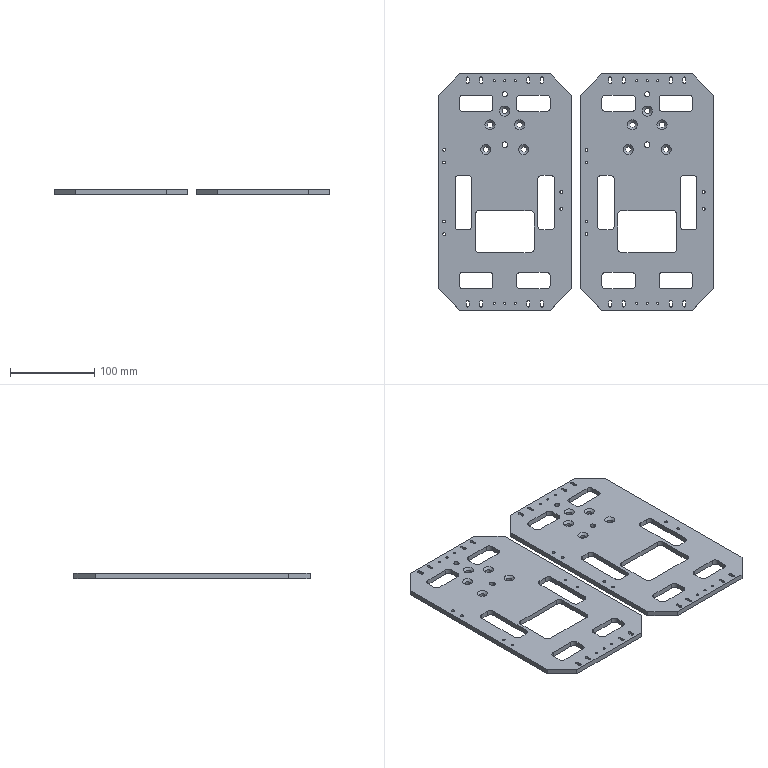Part | 2 solids | 250 faces | box 327 x 280 x 6 mm | volume 398950 mm3 | cylinder 128 | plane 112 | cone 10 | commonest cylinder face diameters 10 x56 3.4 x40 2.5 x12 6.6 x10 6 x6 3.3 x4